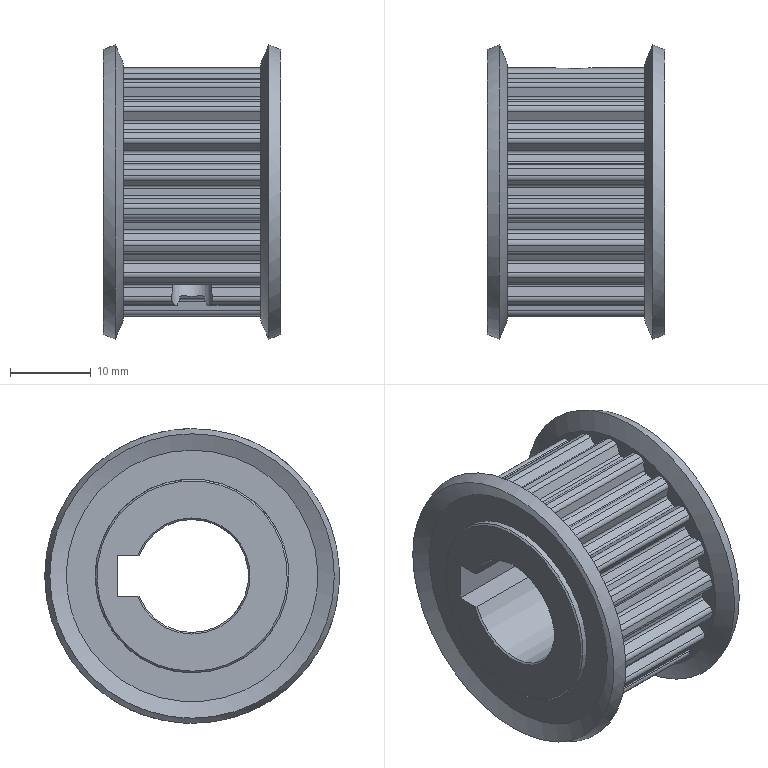Part | NX | 1 solid | 207 faces | box 22 x 36.509 x 36.509 mm | volume 11642 mm3 | cylinder 141 | plane 54 | cone 12 | commonest cylinder face diameters 0.8 x45 1.2 x44 27.4 x22 31 x21 5 x4 4.134 x2